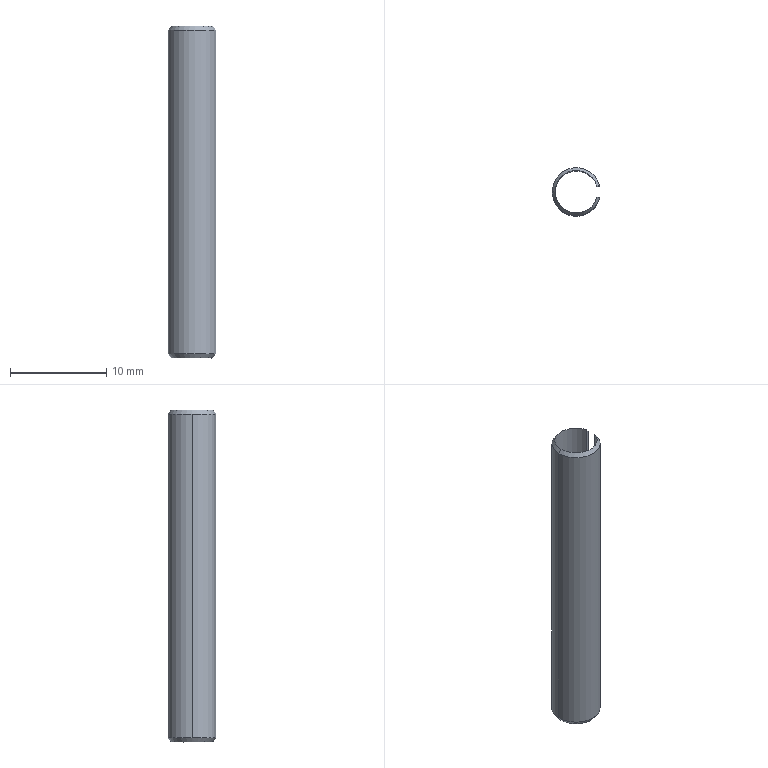Part | STEP file | 103000006354_5×20 | 1 solid | 10 faces | box 4.915 x 5 x 34.44 mm | volume 138.102 mm3 | cone 4 | cylinder 4 | plane 2 | commonest cylinder face diameters 4.4 x2 5 x2
STEP:
#1=CARTESIAN_POINT('',(-2.2,0.,34.72));
#2=VERTEX_POINT('',#1);
#3=CARTESIAN_POINT('',(2.125,-0.5694,34.72));
#4=VERTEX_POINT('',#3);
#5=CARTESIAN_POINT('',(0.,0.,34.72));
#6=DIRECTION('',(0.,0.,-1.));
#7=AXIS2_PLACEMENT_3D('',#5,#6,$);
#8=CIRCLE('',#7,2.2);
#9=EDGE_CURVE('',#2,#4,#8,.F.);
#10=ORIENTED_EDGE('',*,*,#9,.F.);
#11=CARTESIAN_POINT('',(-2.5,0.,34.3));
#12=VERTEX_POINT('',#11);
#13=CARTESIAN_POINT('',(-290620.097,0.,-406830.336));
#14=DIRECTION('',(-0.5812,0.,-0.8137));
#15=VECTOR('',#14,1.);
#16=LINE('',#13,#15);
#17=EDGE_CURVE('',#2,#12,#16,.T.);
#18=ORIENTED_EDGE('',*,*,#17,.T.);
#19=CARTESIAN_POINT('',(2.415,-0.647,34.3));
#20=VERTEX_POINT('',#19);
#21=CARTESIAN_POINT('',(0.,0.,34.3));
#22=DIRECTION('',(0.,0.,-1.));
#23=AXIS2_PLACEMENT_3D('',#21,#22,$);
#24=CIRCLE('',#23,2.5);
#25=EDGE_CURVE('',#20,#12,#24,.T.);
#26=ORIENTED_EDGE('',*,*,#25,.F.);
#27=CARTESIAN_POINT('',(280717.457,-75218.016,-406830.336));
#28=DIRECTION('',(0.5614,-0.1504,-0.8137));
#29=VECTOR('',#28,1.);
#30=LINE('',#27,#29);
#31=EDGE_CURVE('',#20,#4,#30,.F.);
#32=ORIENTED_EDGE('',*,*,#31,.T.);
#33=EDGE_LOOP('',(#10,#18,#26,#32));
#34=FACE_OUTER_BOUND('',#33,.T.);
#35=CARTESIAN_POINT('',(0.,0.,35.));
#36=DIRECTION('',(0.,0.,-1.));
#37=DIRECTION('',(1.,0.,0.));
#38=AXIS2_PLACEMENT_3D('',#35,#36,#37);
#39=CONICAL_SURFACE('',#38,2.,0.6202);
#40=ADVANCED_FACE('',(#34),#39,.T.);
#41=ORIENTED_EDGE('',*,*,#9,.T.);
#42=CARTESIAN_POINT('',(2.125,-0.5694,0.28));
#43=VERTEX_POINT('',#42);
#44=CARTESIAN_POINT('',(2.125,-0.5694,0.));
#45=DIRECTION('',(0.,0.,1.));
#46=VECTOR('',#45,1.);
#47=LINE('',#44,#46);
#48=EDGE_CURVE('',#43,#4,#47,.T.);
#49=ORIENTED_EDGE('',*,*,#48,.F.);
#50=CARTESIAN_POINT('',(-2.2,0.,0.28));
#51=VERTEX_POINT('',#50);
#52=CARTESIAN_POINT('',(2.125,-0.5694,0.28));
#53=CARTESIAN_POINT('',(1.961,-1.181,0.28));
#54=CARTESIAN_POINT('',(1.577,-1.734,0.28));
#55=CARTESIAN_POINT('',(0.9989,-2.12,0.28));
#56=CARTESIAN_POINT('',(-0.3169,-2.407,0.28));
#57=CARTESIAN_POINT('',(-1.514,-1.79,0.28));
#58=CARTESIAN_POINT('',(-1.972,-1.267,0.28));
#59=CARTESIAN_POINT('',(-2.2,-0.6336,0.28));
#60=CARTESIAN_POINT('',(-2.2,0.,0.28));
#61=B_SPLINE_CURVE_WITH_KNOTS('',5,(#52,#53,#54,#55,#56,#57,#58,#59,#60),.UNSPECIFIED.,.F.,.U.,(6,3,6),(-3.168,0.,3.168),.UNSPECIFIED.);
#62=EDGE_CURVE('',#43,#51,#61,.T.);
#63=ORIENTED_EDGE('',*,*,#62,.T.);
#64=CARTESIAN_POINT('',(-2.2,0.,0.));
#65=DIRECTION('',(0.,0.,1.));
#66=VECTOR('',#65,1.);
#67=LINE('',#64,#66);
#68=EDGE_CURVE('',#51,#2,#67,.T.);
#69=ORIENTED_EDGE('',*,*,#68,.T.);
#70=EDGE_LOOP('',(#41,#49,#63,#69));
#71=FACE_OUTER_BOUND('',#70,.T.);
#72=CARTESIAN_POINT('',(0.,0.,0.));
#73=DIRECTION('',(0.,0.,1.));
#74=DIRECTION('',(-1.,0.,0.));
#75=AXIS2_PLACEMENT_3D('',#72,#73,#74);
#76=CYLINDRICAL_SURFACE('',#75,2.2);
#77=ADVANCED_FACE('',(#71),#76,.F.);
#78=ORIENTED_EDGE('',*,*,#17,.F.);
#79=CARTESIAN_POINT('',(2.125,0.5694,34.72));
#80=VERTEX_POINT('',#79);
#81=CARTESIAN_POINT('',(0.,0.,34.72));
#82=DIRECTION('',(0.,0.,-1.));
#83=AXIS2_PLACEMENT_3D('',#81,#82,$);
#84=CIRCLE('',#83,2.2);
#85=EDGE_CURVE('',#80,#2,#84,.F.);
#86=ORIENTED_EDGE('',*,*,#85,.F.);
#87=CARTESIAN_POINT('',(2.415,0.647,34.3));
#88=VERTEX_POINT('',#87);
#89=CARTESIAN_POINT('',(280717.457,75218.016,-406830.336));
#90=DIRECTION('',(0.5614,0.1504,-0.8137));
#91=VECTOR('',#90,1.);
#92=LINE('',#89,#91);
#93=EDGE_CURVE('',#80,#88,#92,.T.);
#94=ORIENTED_EDGE('',*,*,#93,.T.);
#95=CARTESIAN_POINT('',(0.,0.,34.3));
#96=DIRECTION('',(0.,0.,-1.));
#97=AXIS2_PLACEMENT_3D('',#95,#96,$);
#98=CIRCLE('',#97,2.5);
#99=EDGE_CURVE('',#12,#88,#98,.T.);
#100=ORIENTED_EDGE('',*,*,#99,.F.);
#101=EDGE_LOOP('',(#78,#86,#94,#100));
#102=FACE_OUTER_BOUND('',#101,.T.);
#103=CARTESIAN_POINT('',(0.,0.,35.));
#104=DIRECTION('',(0.,0.,-1.));
#105=DIRECTION('',(-1.,0.,0.));
#106=AXIS2_PLACEMENT_3D('',#103,#104,#105);
#107=CONICAL_SURFACE('',#106,2.,0.6202);
#108=ADVANCED_FACE('',(#102),#107,.T.);
#109=ORIENTED_EDGE('',*,*,#25,.T.);
#110=CARTESIAN_POINT('',(-2.5,0.,0.7));
#111=VERTEX_POINT('',#110);
#112=CARTESIAN_POINT('',(-2.5,0.,35.));
#113=DIRECTION('',(0.,0.,-1.));
#114=VECTOR('',#113,1.);
#115=LINE('',#112,#114);
#116=EDGE_CURVE('',#12,#111,#115,.T.);
#117=ORIENTED_EDGE('',*,*,#116,.T.);
#118=CARTESIAN_POINT('',(2.415,-0.647,0.7));
#119=VERTEX_POINT('',#118);
#120=CARTESIAN_POINT('',(0.,0.,0.7));
#121=DIRECTION('',(0.,0.,-1.));
#122=AXIS2_PLACEMENT_3D('',#120,#121,$);
#123=CIRCLE('',#122,2.5);
#124=EDGE_CURVE('',#111,#119,#123,.F.);
#125=ORIENTED_EDGE('',*,*,#124,.T.);
#126=CARTESIAN_POINT('',(2.415,-0.647,35.));
#127=DIRECTION('',(0.,0.,-1.));
#128=VECTOR('',#127,1.);
#129=LINE('',#126,#128);
#130=EDGE_CURVE('',#20,#119,#129,.T.);
#131=ORIENTED_EDGE('',*,*,#130,.F.);
#132=EDGE_LOOP('',(#109,#117,#125,#131));
#133=FACE_OUTER_BOUND('',#132,.T.);
#134=CARTESIAN_POINT('',(0.,0.,35.));
#135=DIRECTION('',(0.,0.,-1.));
#136=DIRECTION('',(1.,0.,0.));
#137=AXIS2_PLACEMENT_3D('',#134,#135,#136);
#138=CYLINDRICAL_SURFACE('',#137,2.5);
#139=ADVANCED_FACE('',(#133),#138,.T.);
#140=ORIENTED_EDGE('',*,*,#130,.T.);
#141=CARTESIAN_POINT('',(2.27,-0.6082,0.49));
#142=DIRECTION('',(0.5614,-0.1504,0.8137));
#143=VECTOR('',#142,1.);
#144=LINE('',#141,#143);
#145=EDGE_CURVE('',#43,#119,#144,.T.);
#146=ORIENTED_EDGE('',*,*,#145,.F.);
#147=ORIENTED_EDGE('',*,*,#48,.T.);
#148=ORIENTED_EDGE('',*,*,#31,.F.);
#149=EDGE_LOOP('',(#140,#146,#147,#148));
#150=FACE_OUTER_BOUND('',#149,.T.);
#151=CARTESIAN_POINT('',(0.,0.,34.72));
#152=DIRECTION('',(0.2588,0.9659,0.));
#153=DIRECTION('',(-0.9659,0.2588,0.));
#154=AXIS2_PLACEMENT_3D('',#151,#152,#153);
#155=PLANE('',#154);
#156=ADVANCED_FACE('',(#150),#155,.T.);
#157=CARTESIAN_POINT('',(-290620.347,0.,406865.686));
#158=DIRECTION('',(-0.5812,0.,0.8137));
#159=VECTOR('',#158,1.);
#160=LINE('',#157,#159);
#161=EDGE_CURVE('',#51,#111,#160,.T.);
#162=ORIENTED_EDGE('',*,*,#161,.F.);
#163=ORIENTED_EDGE('',*,*,#62,.F.);
#164=ORIENTED_EDGE('',*,*,#145,.T.);
#165=ORIENTED_EDGE('',*,*,#124,.F.);
#166=EDGE_LOOP('',(#162,#163,#164,#165));
#167=FACE_OUTER_BOUND('',#166,.T.);
#168=CARTESIAN_POINT('',(0.,0.,0.7));
#169=DIRECTION('',(0.,0.,1.));
#170=DIRECTION('',(-1.,0.,0.));
#171=AXIS2_PLACEMENT_3D('',#168,#169,#170);
#172=CONICAL_SURFACE('',#171,2.5,0.6202);
#173=ADVANCED_FACE('',(#167),#172,.T.);
#174=CARTESIAN_POINT('',(2.125,0.5694,0.28));
#175=VERTEX_POINT('',#174);
#176=CARTESIAN_POINT('',(-2.2,0.,0.28));
#177=CARTESIAN_POINT('',(-2.2,0.6336,0.28));
#178=CARTESIAN_POINT('',(-1.972,1.267,0.28));
#179=CARTESIAN_POINT('',(-1.514,1.79,0.28));
#180=CARTESIAN_POINT('',(-0.3169,2.407,0.28));
#181=CARTESIAN_POINT('',(0.9989,2.12,0.28));
#182=CARTESIAN_POINT('',(1.577,1.734,0.28));
#183=CARTESIAN_POINT('',(1.961,1.181,0.28));
#184=CARTESIAN_POINT('',(2.125,0.5694,0.28));
#185=B_SPLINE_CURVE_WITH_KNOTS('',5,(#176,#177,#178,#179,#180,#181,#182,#183,#184),.UNSPECIFIED.,.F.,.U.,(6,3,6),(-3.168,0.,3.168),.UNSPECIFIED.);
#186=EDGE_CURVE('',#51,#175,#185,.T.);
#187=ORIENTED_EDGE('',*,*,#186,.T.);
#188=CARTESIAN_POINT('',(2.125,0.5694,0.));
#189=DIRECTION('',(0.,0.,1.));
#190=VECTOR('',#189,1.);
#191=LINE('',#188,#190);
#192=EDGE_CURVE('',#80,#175,#191,.F.);
#193=ORIENTED_EDGE('',*,*,#192,.F.);
#194=ORIENTED_EDGE('',*,*,#85,.T.);
#195=ORIENTED_EDGE('',*,*,#68,.F.);
#196=EDGE_LOOP('',(#187,#193,#194,#195));
#197=FACE_OUTER_BOUND('',#196,.T.);
#198=CARTESIAN_POINT('',(0.,0.,0.));
#199=DIRECTION('',(0.,0.,1.));
#200=DIRECTION('',(1.,0.,0.));
#201=AXIS2_PLACEMENT_3D('',#198,#199,#200);
#202=CYLINDRICAL_SURFACE('',#201,2.2);
#203=ADVANCED_FACE('',(#197),#202,.F.);
#204=CARTESIAN_POINT('',(2.415,0.647,0.7));
#205=VERTEX_POINT('',#204);
#206=CARTESIAN_POINT('',(2.415,0.647,17.5));
#207=DIRECTION('',(0.,0.,1.));
#208=VECTOR('',#207,1.);
#209=LINE('',#206,#208);
#210=EDGE_CURVE('',#205,#88,#209,.T.);
#211=ORIENTED_EDGE('',*,*,#210,.T.);
#212=ORIENTED_EDGE('',*,*,#93,.F.);
#213=ORIENTED_EDGE('',*,*,#192,.T.);
#214=CARTESIAN_POINT('',(2.27,0.6082,0.49));
#215=DIRECTION('',(-0.5614,-0.1504,-0.8137));
#216=VECTOR('',#215,1.);
#217=LINE('',#214,#216);
#218=EDGE_CURVE('',#205,#175,#217,.T.);
#219=ORIENTED_EDGE('',*,*,#218,.F.);
#220=EDGE_LOOP('',(#211,#212,#213,#219));
#221=FACE_OUTER_BOUND('',#220,.T.);
#222=CARTESIAN_POINT('',(0.,0.,34.72));
#223=DIRECTION('',(0.2588,-0.9659,0.));
#224=DIRECTION('',(0.9659,0.2588,0.));
#225=AXIS2_PLACEMENT_3D('',#222,#223,#224);
#226=PLANE('',#225);
#227=ADVANCED_FACE('',(#221),#226,.T.);
#228=ORIENTED_EDGE('',*,*,#116,.F.);
#229=ORIENTED_EDGE('',*,*,#99,.T.);
#230=ORIENTED_EDGE('',*,*,#210,.F.);
#231=CARTESIAN_POINT('',(0.,0.,0.7));
#232=DIRECTION('',(0.,0.,-1.));
#233=AXIS2_PLACEMENT_3D('',#231,#232,$);
#234=CIRCLE('',#233,2.5);
#235=EDGE_CURVE('',#205,#111,#234,.F.);
#236=ORIENTED_EDGE('',*,*,#235,.T.);
#237=EDGE_LOOP('',(#228,#229,#230,#236));
#238=FACE_OUTER_BOUND('',#237,.T.);
#239=CARTESIAN_POINT('',(0.,0.,35.));
#240=DIRECTION('',(0.,0.,-1.));
#241=DIRECTION('',(-1.,0.,0.));
#242=AXIS2_PLACEMENT_3D('',#239,#240,#241);
#243=CYLINDRICAL_SURFACE('',#242,2.5);
#244=ADVANCED_FACE('',(#238),#243,.T.);
#245=ORIENTED_EDGE('',*,*,#161,.T.);
#246=ORIENTED_EDGE('',*,*,#235,.F.);
#247=ORIENTED_EDGE('',*,*,#218,.T.);
#248=ORIENTED_EDGE('',*,*,#186,.F.);
#249=EDGE_LOOP('',(#245,#246,#247,#248));
#250=FACE_OUTER_BOUND('',#249,.T.);
#251=CARTESIAN_POINT('',(0.,0.,0.7));
#252=DIRECTION('',(0.,0.,1.));
#253=DIRECTION('',(1.,0.,0.));
#254=AXIS2_PLACEMENT_3D('',#251,#252,#253);
#255=CONICAL_SURFACE('',#254,2.5,0.6202);
#256=ADVANCED_FACE('',(#250),#255,.T.);
#257=CLOSED_SHELL('',(#40,#77,#108,#139,#156,#173,#203,#227,#244,#256));
#258=MANIFOLD_SOLID_BREP('',#257);
#259=(LENGTH_UNIT()NAMED_UNIT(*)SI_UNIT(.MILLI.,.METRE.));
#260=UNCERTAINTY_MEASURE_WITH_UNIT(LENGTH_MEASURE(0.005),#259,'','');
#261=(NAMED_UNIT(*)PLANE_ANGLE_UNIT()SI_UNIT($,.RADIAN.));
#262=(NAMED_UNIT(*)SI_UNIT($,.STERADIAN.)SOLID_ANGLE_UNIT());
#263=(GEOMETRIC_REPRESENTATION_CONTEXT(3)GLOBAL_UNCERTAINTY_ASSIGNED_CONTEXT((#260))GLOBAL_UNIT_ASSIGNED_CONTEXT((#259,#261,#262))REPRESENTATION_CONTEXT('',''));
#264=ADVANCED_BREP_SHAPE_REPRESENTATION('',(#258),#263);